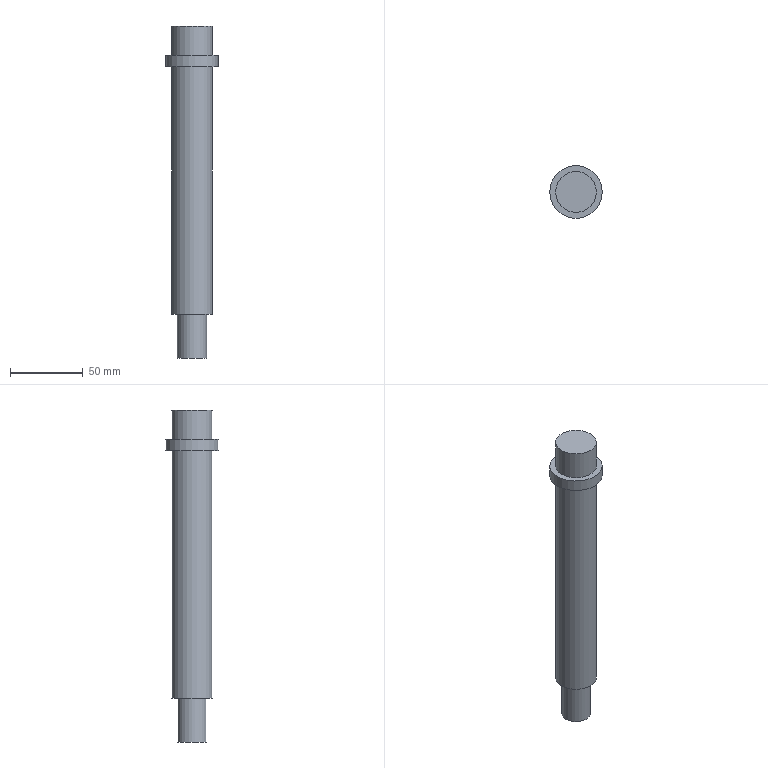Part | NX | features solid 2 | 1 solid | 9 faces | box 36 x 36 x 228 mm | volume 134561 mm3 | plane 5 | cylinder 4 | commonest cylinder face diameters 28 x2 20 x1 36 x1
STEP:
#1=CARTESIAN_POINT('',(-805.,455.,-380.));
#2=VERTEX_POINT('',#1);
#3=CARTESIAN_POINT('',(-795.,455.,-380.));
#4=DIRECTION('',(0.,0.,1.));
#5=DIRECTION('',(-1.,0.,0.));
#6=AXIS2_PLACEMENT_3D('',#3,#4,#5);
#7=CIRCLE('',#6,10.);
#8=EDGE_CURVE('',#2,#2,#7,.T.);
#9=ORIENTED_EDGE('',*,*,#8,.T.);
#10=EDGE_LOOP('',(#9));
#11=FACE_BOUND('',#10,.T.);
#12=CARTESIAN_POINT('',(-781.,455.,-380.));
#13=VERTEX_POINT('',#12);
#14=CARTESIAN_POINT('',(-795.,455.,-380.));
#15=DIRECTION('',(0.,0.,-1.));
#16=DIRECTION('',(1.,0.,0.));
#17=AXIS2_PLACEMENT_3D('',#14,#15,#16);
#18=CIRCLE('',#17,14.);
#19=EDGE_CURVE('',#13,#13,#18,.T.);
#20=ORIENTED_EDGE('',*,*,#19,.T.);
#21=EDGE_LOOP('',(#20));
#22=FACE_BOUND('',#21,.T.);
#23=CARTESIAN_POINT('',(-795.,455.,-380.));
#24=DIRECTION('',(0.,0.,-1.));
#25=DIRECTION('',(1.,0.,0.));
#26=AXIS2_PLACEMENT_3D('',#23,#24,#25);
#27=PLANE('',#26);
#28=ADVANCED_FACE('',(#11,#22),#27,.T.);
#29=CARTESIAN_POINT('',(-809.,455.,-210.));
#30=VERTEX_POINT('',#29);
#31=CARTESIAN_POINT('',(-795.,455.,-210.));
#32=DIRECTION('',(0.,0.,-1.));
#33=DIRECTION('',(-1.,0.,0.));
#34=AXIS2_PLACEMENT_3D('',#31,#32,#33);
#35=CIRCLE('',#34,14.);
#36=EDGE_CURVE('',#30,#30,#35,.T.);
#37=ORIENTED_EDGE('',*,*,#36,.T.);
#38=EDGE_LOOP('',(#37));
#39=FACE_BOUND('',#38,.T.);
#40=ORIENTED_EDGE('',*,*,#19,.F.);
#41=EDGE_LOOP('',(#40));
#42=FACE_BOUND('',#41,.T.);
#43=CARTESIAN_POINT('',(-795.,455.,-380.));
#44=DIRECTION('',(0.,0.,1.));
#45=DIRECTION('',(-1.,0.,0.));
#46=AXIS2_PLACEMENT_3D('',#43,#44,#45);
#47=CYLINDRICAL_SURFACE('',#46,14.);
#48=ADVANCED_FACE('',(#39,#42),#47,.T.);
#49=CARTESIAN_POINT('',(-785.,455.,-410.));
#50=VERTEX_POINT('',#49);
#51=CARTESIAN_POINT('',(-795.,455.,-410.));
#52=DIRECTION('',(0.,0.,-1.));
#53=DIRECTION('',(1.,0.,0.));
#54=AXIS2_PLACEMENT_3D('',#51,#52,#53);
#55=CIRCLE('',#54,10.);
#56=EDGE_CURVE('',#50,#50,#55,.T.);
#57=ORIENTED_EDGE('',*,*,#56,.T.);
#58=EDGE_LOOP('',(#57));
#59=FACE_BOUND('',#58,.T.);
#60=CARTESIAN_POINT('',(-795.,455.,-410.));
#61=DIRECTION('',(0.,0.,-1.));
#62=DIRECTION('',(1.,0.,0.));
#63=AXIS2_PLACEMENT_3D('',#60,#61,#62);
#64=PLANE('',#63);
#65=ADVANCED_FACE('',(#59),#64,.T.);
#66=ORIENTED_EDGE('',*,*,#56,.F.);
#67=EDGE_LOOP('',(#66));
#68=FACE_BOUND('',#67,.T.);
#69=ORIENTED_EDGE('',*,*,#8,.F.);
#70=EDGE_LOOP('',(#69));
#71=FACE_BOUND('',#70,.T.);
#72=CARTESIAN_POINT('',(-795.,455.,-380.));
#73=DIRECTION('',(0.,0.,-1.));
#74=DIRECTION('',(1.,0.,0.));
#75=AXIS2_PLACEMENT_3D('',#72,#73,#74);
#76=CYLINDRICAL_SURFACE('',#75,10.);
#77=ADVANCED_FACE('',(#68,#71),#76,.T.);
#78=CARTESIAN_POINT('',(-781.,455.,-202.));
#79=VERTEX_POINT('',#78);
#80=CARTESIAN_POINT('',(-795.,455.,-202.));
#81=DIRECTION('',(0.,0.,-1.));
#82=DIRECTION('',(1.,0.,0.));
#83=AXIS2_PLACEMENT_3D('',#80,#81,#82);
#84=CIRCLE('',#83,14.);
#85=EDGE_CURVE('',#79,#79,#84,.T.);
#86=ORIENTED_EDGE('',*,*,#85,.T.);
#87=EDGE_LOOP('',(#86));
#88=FACE_BOUND('',#87,.T.);
#89=CARTESIAN_POINT('',(-813.,455.,-202.));
#90=VERTEX_POINT('',#89);
#91=CARTESIAN_POINT('',(-795.,455.,-202.));
#92=DIRECTION('',(0.,0.,1.));
#93=DIRECTION('',(-1.,0.,0.));
#94=AXIS2_PLACEMENT_3D('',#91,#92,#93);
#95=CIRCLE('',#94,18.);
#96=EDGE_CURVE('',#90,#90,#95,.T.);
#97=ORIENTED_EDGE('',*,*,#96,.T.);
#98=EDGE_LOOP('',(#97));
#99=FACE_BOUND('',#98,.T.);
#100=CARTESIAN_POINT('',(-795.,455.,-202.));
#101=DIRECTION('',(0.,0.,1.));
#102=DIRECTION('',(-1.,0.,0.));
#103=AXIS2_PLACEMENT_3D('',#100,#101,#102);
#104=PLANE('',#103);
#105=ADVANCED_FACE('',(#88,#99),#104,.T.);
#106=ORIENTED_EDGE('',*,*,#36,.F.);
#107=EDGE_LOOP('',(#106));
#108=FACE_BOUND('',#107,.T.);
#109=CARTESIAN_POINT('',(-777.,455.,-210.));
#110=VERTEX_POINT('',#109);
#111=CARTESIAN_POINT('',(-795.,455.,-210.));
#112=DIRECTION('',(0.,0.,-1.));
#113=DIRECTION('',(1.,0.,0.));
#114=AXIS2_PLACEMENT_3D('',#111,#112,#113);
#115=CIRCLE('',#114,18.);
#116=EDGE_CURVE('',#110,#110,#115,.T.);
#117=ORIENTED_EDGE('',*,*,#116,.T.);
#118=EDGE_LOOP('',(#117));
#119=FACE_BOUND('',#118,.T.);
#120=CARTESIAN_POINT('',(-795.,455.,-210.));
#121=DIRECTION('',(0.,0.,-1.));
#122=DIRECTION('',(1.,0.,0.));
#123=AXIS2_PLACEMENT_3D('',#120,#121,#122);
#124=PLANE('',#123);
#125=ADVANCED_FACE('',(#108,#119),#124,.T.);
#126=ORIENTED_EDGE('',*,*,#96,.F.);
#127=EDGE_LOOP('',(#126));
#128=FACE_BOUND('',#127,.T.);
#129=ORIENTED_EDGE('',*,*,#116,.F.);
#130=EDGE_LOOP('',(#129));
#131=FACE_BOUND('',#130,.T.);
#132=CARTESIAN_POINT('',(-795.,455.,-210.));
#133=DIRECTION('',(0.,0.,1.));
#134=DIRECTION('',(-1.,0.,0.));
#135=AXIS2_PLACEMENT_3D('',#132,#133,#134);
#136=CYLINDRICAL_SURFACE('',#135,18.);
#137=ADVANCED_FACE('',(#128,#131),#136,.T.);
#138=CARTESIAN_POINT('',(-809.,455.,-182.));
#139=VERTEX_POINT('',#138);
#140=CARTESIAN_POINT('',(-795.,455.,-182.));
#141=DIRECTION('',(0.,0.,1.));
#142=DIRECTION('',(-1.,0.,0.));
#143=AXIS2_PLACEMENT_3D('',#140,#141,#142);
#144=CIRCLE('',#143,14.);
#145=EDGE_CURVE('',#139,#139,#144,.T.);
#146=ORIENTED_EDGE('',*,*,#145,.T.);
#147=EDGE_LOOP('',(#146));
#148=FACE_BOUND('',#147,.T.);
#149=CARTESIAN_POINT('',(-795.,455.,-182.));
#150=DIRECTION('',(0.,0.,1.));
#151=DIRECTION('',(-1.,0.,0.));
#152=AXIS2_PLACEMENT_3D('',#149,#150,#151);
#153=PLANE('',#152);
#154=ADVANCED_FACE('',(#148),#153,.T.);
#155=ORIENTED_EDGE('',*,*,#145,.F.);
#156=EDGE_LOOP('',(#155));
#157=FACE_BOUND('',#156,.T.);
#158=ORIENTED_EDGE('',*,*,#85,.F.);
#159=EDGE_LOOP('',(#158));
#160=FACE_BOUND('',#159,.T.);
#161=CARTESIAN_POINT('',(-795.,455.,-202.));
#162=DIRECTION('',(0.,0.,1.));
#163=DIRECTION('',(-1.,0.,0.));
#164=AXIS2_PLACEMENT_3D('',#161,#162,#163);
#165=CYLINDRICAL_SURFACE('',#164,14.);
#166=ADVANCED_FACE('',(#157,#160),#165,.T.);
#167=CLOSED_SHELL('',(#28,#48,#65,#77,#105,#125,#137,#154,#166));
#168=MANIFOLD_SOLID_BREP('',#167);
#169=(LENGTH_UNIT()NAMED_UNIT(*)SI_UNIT(.MILLI.,.METRE.));
#170=UNCERTAINTY_MEASURE_WITH_UNIT(LENGTH_MEASURE(0.00001),#169,'','');
#171=(NAMED_UNIT(*)PLANE_ANGLE_UNIT()SI_UNIT($,.RADIAN.));
#172=(NAMED_UNIT(*)SI_UNIT($,.STERADIAN.)SOLID_ANGLE_UNIT());
#173=(GEOMETRIC_REPRESENTATION_CONTEXT(3)GLOBAL_UNCERTAINTY_ASSIGNED_CONTEXT((#170))GLOBAL_UNIT_ASSIGNED_CONTEXT((#169,#171,#172))REPRESENTATION_CONTEXT('',''));
#174=ADVANCED_BREP_SHAPE_REPRESENTATION('',(#168),#173);